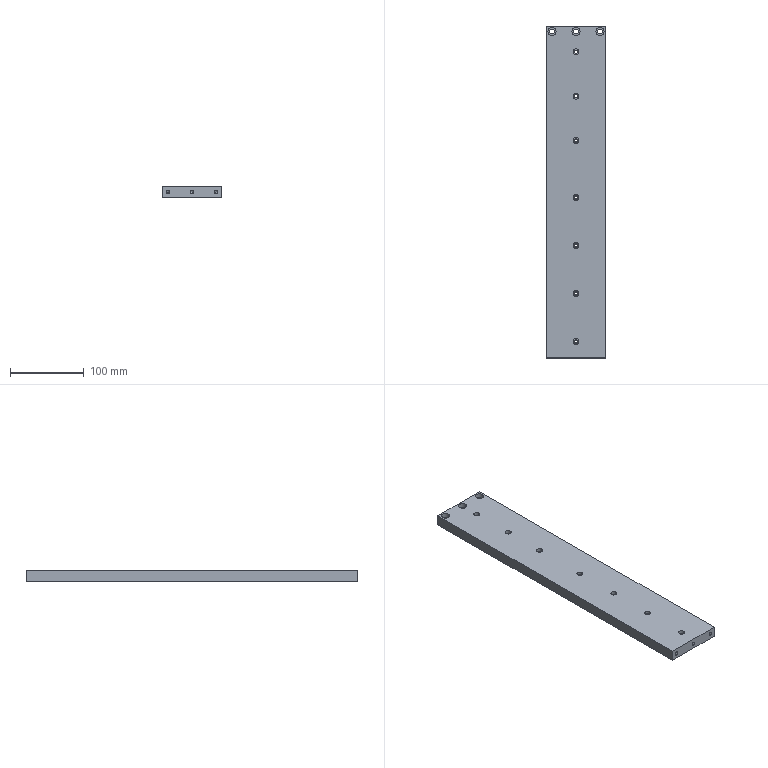Part | SolidWorks | features HoleWzd 4, Extrusion 1 | 1 solid | 68 faces | box 80 x 450 x 15 mm | volume 533651 mm3 | cylinder 46 | plane 16 | cone 6 | commonest cylinder face diameters 4.5 x14 8 x14 5 x6 6.6 x6 11 x6